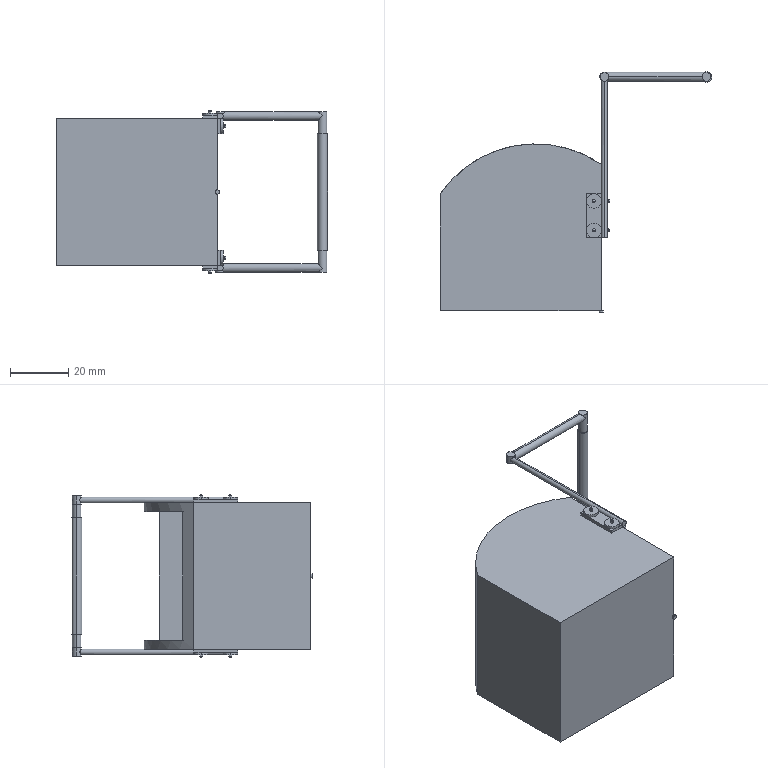Part | SolidWorks | features ICE 22, Fillet 5, Extrusion 1, Shell 1 | 2 solids | 138 faces | box 92.75 x 82.25 x 56 mm | volume 38055 mm3 | plane 66 | cylinder 56 | sphere 16 | commonest cylinder face diameters 1 x16 5 x16 3 x15 2 x4 1.5 x2 3.5 x2